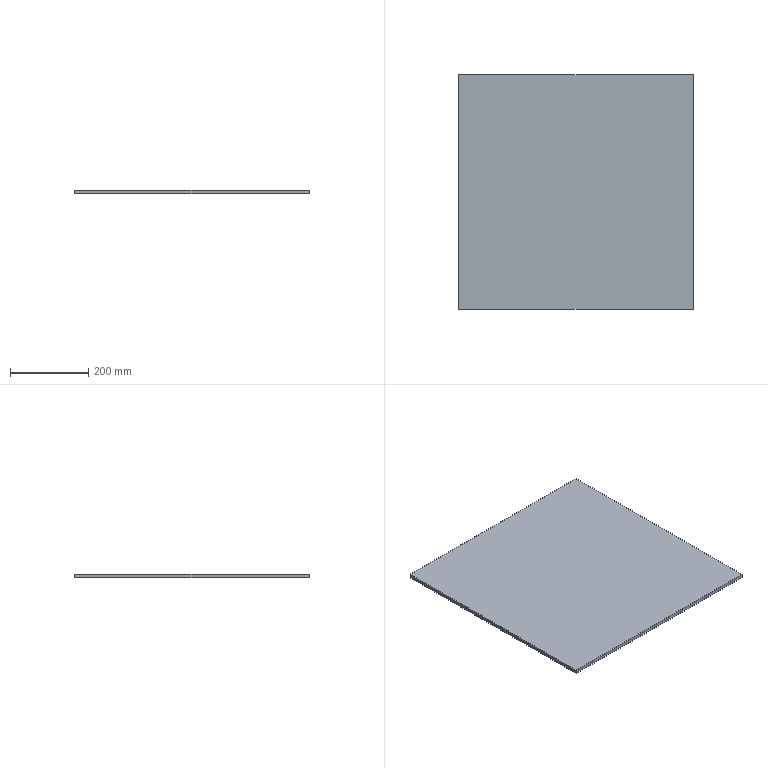Part | SolidWorks | features Extrusion 1 | 1 solid | 6 faces | box 600 x 600 x 10 mm | volume 3600000 mm3 | plane 6
STEP:
#1=CARTESIAN_POINT('',(0.,600.,0.));
#2=VERTEX_POINT('',#1);
#3=CARTESIAN_POINT('',(0.,0.,0.));
#4=VERTEX_POINT('',#3);
#5=CARTESIAN_POINT('',(0.,0.,0.));
#6=DIRECTION('',(0.,-1.,0.));
#7=VECTOR('',#6,1000.);
#8=LINE('',#5,#7);
#9=EDGE_CURVE('',#2,#4,#8,.T.);
#10=ORIENTED_EDGE('',*,*,#9,.T.);
#11=CARTESIAN_POINT('',(0.,0.,10.));
#12=VERTEX_POINT('',#11);
#13=CARTESIAN_POINT('',(0.,0.,10.));
#14=DIRECTION('',(0.,0.,-1.));
#15=VECTOR('',#14,1000.);
#16=LINE('',#13,#15);
#17=EDGE_CURVE('',#12,#4,#16,.T.);
#18=ORIENTED_EDGE('',*,*,#17,.F.);
#19=CARTESIAN_POINT('',(0.,600.,10.));
#20=VERTEX_POINT('',#19);
#21=CARTESIAN_POINT('',(0.,0.,10.));
#22=DIRECTION('',(0.,-1.,0.));
#23=VECTOR('',#22,1000.);
#24=LINE('',#21,#23);
#25=EDGE_CURVE('',#20,#12,#24,.T.);
#26=ORIENTED_EDGE('',*,*,#25,.F.);
#27=CARTESIAN_POINT('',(0.,600.,10.));
#28=DIRECTION('',(0.,0.,-1.));
#29=VECTOR('',#28,1000.);
#30=LINE('',#27,#29);
#31=EDGE_CURVE('',#20,#2,#30,.T.);
#32=ORIENTED_EDGE('',*,*,#31,.T.);
#33=EDGE_LOOP('',(#10,#18,#26,#32));
#34=FACE_OUTER_BOUND('',#33,.T.);
#35=CARTESIAN_POINT('',(0.,0.,10.));
#36=DIRECTION('',(1.,0.,0.));
#37=DIRECTION('',(0.,0.,-1.));
#38=AXIS2_PLACEMENT_3D('',#35,#36,#37);
#39=PLANE('',#38);
#40=ADVANCED_FACE('',(#34),#39,.F.);
#41=CARTESIAN_POINT('',(600.,0.,0.));
#42=VERTEX_POINT('',#41);
#43=CARTESIAN_POINT('',(0.,0.,0.));
#44=DIRECTION('',(1.,0.,0.));
#45=VECTOR('',#44,1000.);
#46=LINE('',#43,#45);
#47=EDGE_CURVE('',#4,#42,#46,.T.);
#48=ORIENTED_EDGE('',*,*,#47,.T.);
#49=CARTESIAN_POINT('',(600.,0.,10.));
#50=VERTEX_POINT('',#49);
#51=CARTESIAN_POINT('',(600.,0.,10.));
#52=DIRECTION('',(0.,0.,-1.));
#53=VECTOR('',#52,1000.);
#54=LINE('',#51,#53);
#55=EDGE_CURVE('',#50,#42,#54,.T.);
#56=ORIENTED_EDGE('',*,*,#55,.F.);
#57=CARTESIAN_POINT('',(0.,0.,10.));
#58=DIRECTION('',(1.,0.,0.));
#59=VECTOR('',#58,1000.);
#60=LINE('',#57,#59);
#61=EDGE_CURVE('',#12,#50,#60,.T.);
#62=ORIENTED_EDGE('',*,*,#61,.F.);
#63=ORIENTED_EDGE('',*,*,#17,.T.);
#64=EDGE_LOOP('',(#48,#56,#62,#63));
#65=FACE_OUTER_BOUND('',#64,.T.);
#66=CARTESIAN_POINT('',(0.,0.,10.));
#67=DIRECTION('',(0.,1.,0.));
#68=DIRECTION('',(0.,0.,1.));
#69=AXIS2_PLACEMENT_3D('',#66,#67,#68);
#70=PLANE('',#69);
#71=ADVANCED_FACE('',(#65),#70,.F.);
#72=CARTESIAN_POINT('',(600.,600.,0.));
#73=VERTEX_POINT('',#72);
#74=CARTESIAN_POINT('',(600.,0.,0.));
#75=DIRECTION('',(0.,1.,0.));
#76=VECTOR('',#75,1000.);
#77=LINE('',#74,#76);
#78=EDGE_CURVE('',#42,#73,#77,.T.);
#79=ORIENTED_EDGE('',*,*,#78,.T.);
#80=CARTESIAN_POINT('',(600.,600.,10.));
#81=VERTEX_POINT('',#80);
#82=CARTESIAN_POINT('',(600.,600.,10.));
#83=DIRECTION('',(0.,0.,-1.));
#84=VECTOR('',#83,1000.);
#85=LINE('',#82,#84);
#86=EDGE_CURVE('',#81,#73,#85,.T.);
#87=ORIENTED_EDGE('',*,*,#86,.F.);
#88=CARTESIAN_POINT('',(600.,0.,10.));
#89=DIRECTION('',(0.,1.,0.));
#90=VECTOR('',#89,1000.);
#91=LINE('',#88,#90);
#92=EDGE_CURVE('',#50,#81,#91,.T.);
#93=ORIENTED_EDGE('',*,*,#92,.F.);
#94=ORIENTED_EDGE('',*,*,#55,.T.);
#95=EDGE_LOOP('',(#79,#87,#93,#94));
#96=FACE_OUTER_BOUND('',#95,.T.);
#97=CARTESIAN_POINT('',(600.,0.,10.));
#98=DIRECTION('',(-1.,0.,0.));
#99=DIRECTION('',(0.,0.,1.));
#100=AXIS2_PLACEMENT_3D('',#97,#98,#99);
#101=PLANE('',#100);
#102=ADVANCED_FACE('',(#96),#101,.F.);
#103=CARTESIAN_POINT('',(0.,600.,0.));
#104=DIRECTION('',(-1.,0.,0.));
#105=VECTOR('',#104,1000.);
#106=LINE('',#103,#105);
#107=EDGE_CURVE('',#73,#2,#106,.T.);
#108=ORIENTED_EDGE('',*,*,#107,.T.);
#109=ORIENTED_EDGE('',*,*,#31,.F.);
#110=CARTESIAN_POINT('',(0.,600.,10.));
#111=DIRECTION('',(-1.,0.,0.));
#112=VECTOR('',#111,1000.);
#113=LINE('',#110,#112);
#114=EDGE_CURVE('',#81,#20,#113,.T.);
#115=ORIENTED_EDGE('',*,*,#114,.F.);
#116=ORIENTED_EDGE('',*,*,#86,.T.);
#117=EDGE_LOOP('',(#108,#109,#115,#116));
#118=FACE_OUTER_BOUND('',#117,.T.);
#119=CARTESIAN_POINT('',(0.,600.,10.));
#120=DIRECTION('',(0.,-1.,0.));
#121=DIRECTION('',(0.,0.,-1.));
#122=AXIS2_PLACEMENT_3D('',#119,#120,#121);
#123=PLANE('',#122);
#124=ADVANCED_FACE('',(#118),#123,.F.);
#125=ORIENTED_EDGE('',*,*,#25,.T.);
#126=ORIENTED_EDGE('',*,*,#61,.T.);
#127=ORIENTED_EDGE('',*,*,#92,.T.);
#128=ORIENTED_EDGE('',*,*,#114,.T.);
#129=EDGE_LOOP('',(#125,#126,#127,#128));
#130=FACE_OUTER_BOUND('',#129,.T.);
#131=CARTESIAN_POINT('',(0.,0.,10.));
#132=DIRECTION('',(0.,0.,-1.));
#133=DIRECTION('',(-1.,0.,0.));
#134=AXIS2_PLACEMENT_3D('',#131,#132,#133);
#135=PLANE('',#134);
#136=ADVANCED_FACE('',(#130),#135,.F.);
#137=ORIENTED_EDGE('',*,*,#9,.F.);
#138=ORIENTED_EDGE('',*,*,#107,.F.);
#139=ORIENTED_EDGE('',*,*,#78,.F.);
#140=ORIENTED_EDGE('',*,*,#47,.F.);
#141=EDGE_LOOP('',(#137,#138,#139,#140));
#142=FACE_OUTER_BOUND('',#141,.T.);
#143=CARTESIAN_POINT('',(0.,0.,0.));
#144=DIRECTION('',(0.,0.,-1.));
#145=DIRECTION('',(-1.,0.,0.));
#146=AXIS2_PLACEMENT_3D('',#143,#144,#145);
#147=PLANE('',#146);
#148=ADVANCED_FACE('',(#142),#147,.T.);
#149=CLOSED_SHELL('',(#40,#71,#102,#124,#136,#148));
#150=MANIFOLD_SOLID_BREP('',#149);
#151=CARTESIAN_POINT('',(0.,0.,0.));
#152=DIRECTION('',(0.,0.,1.));
#153=DIRECTION('',(1.,0.,0.));
#154=AXIS2_PLACEMENT_3D('',#151,#152,#153);
#155=(LENGTH_UNIT()NAMED_UNIT(*)SI_UNIT(.MILLI.,.METRE.));
#156=UNCERTAINTY_MEASURE_WITH_UNIT(LENGTH_MEASURE(0.00001),#155,'','');
#157=(NAMED_UNIT(*)PLANE_ANGLE_UNIT()SI_UNIT($,.RADIAN.));
#158=(NAMED_UNIT(*)SI_UNIT($,.STERADIAN.)SOLID_ANGLE_UNIT());
#159=(GEOMETRIC_REPRESENTATION_CONTEXT(3)GLOBAL_UNCERTAINTY_ASSIGNED_CONTEXT((#156))GLOBAL_UNIT_ASSIGNED_CONTEXT((#155,#157,#158))REPRESENTATION_CONTEXT('',''));
#160=ADVANCED_BREP_SHAPE_REPRESENTATION('',(#150,#154),#159);